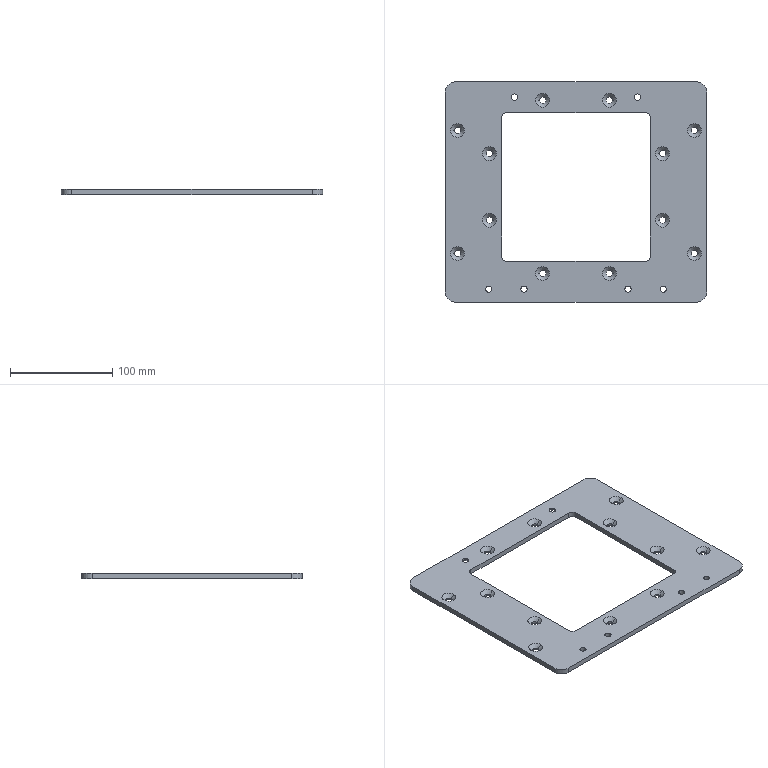NC program | NX | posted with a generic post | part box 255 x 215 x 5 mm
Lines 6275 to 7663 of 7663:
(ZLEVEL_PROFILE_COPY_1_COPY_2 , TOOL : D10JING)
N12512 T14 M6
N12514 G54
N12516 G17 G0 G90 X67.5 Y13.343 S9500 M3
N12518 G43 Z30. H14
N12520 Z1.5
N12522 G94 G1 Y72.494 Z-1.6 F1000.
N12524 X67.454 Y72.5 F1500.
N12526 X-67.41
N12528 X-67.5 Y72.494
N12530 Y-62.41
N12532 X-67.494 Y-62.5
N12534 X67.494
N12536 X67.5 Y-62.454
N12538 Y72.494
N12540 X62.661 Y72.5 Z-1.614
N12542 X-57.777 Z-1.971
N12544 X-62.593 Z-1.985
N12546 X-67.41 Y72.498 Z-2.
N12548 X-67.491 Y72.493
N12550 X-67.496 Y72.424
N12552 X-67.5 Y67.643 Z-2.014
N12554 Y62.858 Z-2.029
N12556 Y-52.774 Z-2.371
N12558 Y-57.592 Z-2.385
N12560 X-67.498 Y-62.41 Z-2.4
N12562 X-67.493 Y-62.491
N12564 X-67.424 Y-62.496
N12566 X-62.64 Y-62.5 Z-2.414
N12568 X-57.852 Z-2.429
N12570 X57.852 Z-2.771
N12572 X62.653 Z-2.786
N12574 X67.492 Y-62.492 Z-2.8
N12576 X67.5 Y-57.635 Z-2.814
N12578 Y-52.815 Z-2.829
N12580 Y67.675 Z-3.186
N12582 Y72.494 Z-3.2
N12584 X62.661 Y72.5 Z-3.214
N12586 X-57.777 Z-3.571
N12588 X-62.593 Z-3.585
N12590 X-67.41 Y72.498 Z-3.6
N12592 X-67.491 Y72.493
N12594 X-67.496 Y72.424
N12596 X-67.5 Y67.643 Z-3.614
N12598 Y62.858 Z-3.629
N12600 Y-52.774 Z-3.971
N12602 Y-57.592 Z-3.985
N12604 X-67.498 Y-62.41 Z-4.
N12606 X-67.493 Y-62.491
N12608 X-67.424 Y-62.496
N12610 X-62.64 Y-62.5 Z-4.014
N12612 X-57.852 Z-4.029
N12614 X57.852 Z-4.371
N12616 X62.653 Z-4.386
N12618 X67.493 Y-62.493 Z-4.4
N12620 X67.5 Y-57.635 Z-4.414
N12622 Y-52.815 Z-4.429
N12624 Y62.855 Z-4.771
N12626 Y67.675 Z-4.786
N12628 Y72.494 Z-4.8
N12630 X67.454 Y72.5
N12632 X-67.41
N12634 X-67.5 Y72.494
N12636 Y-62.41
N12638 X-67.494 Y-62.5
N12640 X67.494
N12642 X67.5 Y-62.454
N12644 Y72.494
N12646 Z-3.3
N12648 G0 Z30.
(ZLEVEL_PROFILE_COPY_1_COPY_COPY , TOOL : D10JING)
N12650 X-119.184 Y114.416
N12652 Z-3.525
N12654 G1 Z-4.525 F1000.
N12656 X-118.366 Y113.
N12658 G3 X-117.5 Y112.5 R1.
N12660 G1 X117.5 F1200.
N12662 G2 X132.5 Y97.5 R15.
N12664 G1 Y-97.5
N12666 G2 X117.5 Y-112.5 R15.
N12668 G1 X-117.5
N12670 G2 X-132.5 Y-97.5 R15.
N12672 G1 Y97.5
N12674 G2 X-117.5 Y112.5 R15.
N12676 G1 X117.43 Z-4.556
N12678 X117.653 Y112.499
N12680 X117.877 Y112.495
N12682 X118.1 Y112.488
N12684 X118.323 Y112.477
N12686 X118.546 Y112.463
N12688 X118.769 Y112.446
N12690 X118.992 Y112.426
N12692 X119.214 Y112.402
N12694 X119.436 Y112.375
N12696 X119.657 Y112.344
N12698 X119.878 Y112.31
N12700 X120.099 Y112.273
N12702 X120.319 Y112.233
N12704 X120.538 Y112.189
N12706 X120.756 Y112.142
N12708 X120.974 Y112.092
N12710 X121.191 Y112.039
N12712 X121.408 Y111.982
N12714 X121.623 Y111.922
N12716 X121.837 Y111.859
N12718 X122.051 Y111.793
N12720 X122.263 Y111.724
N12722 X122.475 Y111.651
N12724 X122.685 Y111.575
N12726 X122.894 Y111.497 Z-4.557
N12728 X123.102 Y111.415
N12730 X123.309 Y111.33
N12732 X123.514 Y111.241
N12734 X123.718 Y111.15
N12736 X123.921 Y111.056
N12738 X124.122 Y110.959
N12740 X124.322 Y110.859
N12742 X124.521 Y110.756
N12744 X124.717 Y110.65
N12746 X124.912 Y110.541
N12748 X125.106 Y110.429
N12750 X125.298 Y110.314
N12752 X125.488 Y110.196
N12754 X125.676 Y110.076
N12756 X125.863 Y109.953
N12758 X126.047 Y109.827
N12760 X126.23 Y109.698
N12762 X126.411 Y109.566
N12764 X126.59 Y109.432
N12766 X126.766 Y109.295
N12768 X126.941 Y109.156
N12770 X127.114 Y109.014
N12772 X127.284 Y108.87
N12774 X127.453 Y108.722
N12776 X127.619 Y108.573
N12778 X127.783 Y108.421
N12780 X127.944 Y108.266
N12782 X128.104 Y108.11
N12784 X128.26 Y107.95
N12786 X128.415 Y107.789
N12788 X128.567 Y107.625
N12790 X128.717 Y107.459
N12792 X128.864 Y107.291
N12794 X129.009 Y107.12 Z-4.558
N12796 X129.151 Y106.948
N12798 X129.29 Y106.773
N12800 X129.427 Y106.597
N12802 X129.561 Y106.418
N12804 X129.693 Y106.237
N12806 X129.822 Y106.054
N12808 X129.948 Y105.87
N12810 X130.071 Y105.683
N12812 X130.192 Y105.495
N12814 X130.309 Y105.305
N12816 X130.424 Y105.113
N12818 X130.536 Y104.92
N12820 X130.645 Y104.725
N12822 X130.752 Y104.528
N12824 X130.855 Y104.33
N12826 X130.955 Y104.13
N12828 X131.052 Y103.929
N12830 X131.147 Y103.726
N12832 X131.238 Y103.522
N12834 X131.326 Y103.317
N12836 X131.411 Y103.11
N12838 X131.493 Y102.902
N12840 X131.572 Y102.693
N12842 X131.648 Y102.483
N12844 X131.721 Y102.272
N12846 X131.79 Y102.059
N12848 X131.857 Y101.846
N12850 X131.92 Y101.631
N12852 X131.98 Y101.416
N12854 X132.037 Y101.2
N12856 X132.09 Y100.983
N12858 X132.14 Y100.765
N12860 X132.187 Y100.546
N12862 X132.231 Y100.327
N12864 X132.272 Y100.107 Z-4.559
N12866 X132.309 Y99.887
N12868 X132.343 Y99.666
N12870 X132.373 Y99.444
N12872 X132.401 Y99.223
N12874 X132.425 Y99.
N12876 X132.445 Y98.778
N12878 X132.463 Y98.555
N12880 X132.477 Y98.332
N12882 X132.488 Y98.109
N12884 X132.495 Y97.885
N12886 X132.499 Y97.662
N12888 X132.5 Y97.438
N12890 Y-97.48 Z-4.584
N12892 X132.499 Y-97.703
N12894 X132.494 Y-97.927
N12896 X132.486 Y-98.15
N12898 X132.475 Y-98.373 Z-4.585
N12900 X132.46 Y-98.596
N12902 X132.442 Y-98.819
N12904 X132.421 Y-99.042
N12906 X132.396 Y-99.264
N12908 X132.368 Y-99.485
N12910 X132.337 Y-99.707
N12912 X132.302 Y-99.928
N12914 X132.264 Y-100.148
N12916 X132.223 Y-100.368
N12918 X132.179 Y-100.587
N12920 X132.131 Y-100.805
N12922 X132.08 Y-101.023
N12924 X132.026 Y-101.24
N12926 X131.969 Y-101.456
N12928 X131.908 Y-101.671
N12930 X131.845 Y-101.885
N12932 X131.778 Y-102.098
N12934 X131.708 Y-102.311
N12936 X131.634 Y-102.522
N12938 X131.558 Y-102.732
N12940 X131.478 Y-102.941
N12942 X131.396 Y-103.149
N12944 X131.31 Y-103.355
N12946 X131.221 Y-103.56
N12948 X131.13 Y-103.764
N12950 X131.035 Y-103.966
N12952 X130.937 Y-104.167
N12954 X130.836 Y-104.367
N12956 X130.732 Y-104.565
N12958 X130.625 Y-104.761
N12960 X130.516 Y-104.956
N12962 X130.403 Y-105.149
N12964 X130.288 Y-105.34
N12966 X130.17 Y-105.53 Z-4.586
N12968 X130.048 Y-105.718
N12970 X129.925 Y-105.904
N12972 X129.798 Y-106.088
N12974 X129.669 Y-106.271
N12976 X129.537 Y-106.451
N12978 X129.402 Y-106.629
N12980 X129.265 Y-106.806
N12982 X129.125 Y-106.98
N12984 X128.982 Y-107.152
N12986 X128.837 Y-107.322
N12988 X128.689 Y-107.49
N12990 X128.539 Y-107.656
N12992 X128.387 Y-107.819
N12994 X128.232 Y-107.98
N12996 X128.074 Y-108.139
N12998 X127.915 Y-108.295
N13000 X127.753 Y-108.449
N13002 X127.588 Y-108.601
N13004 X127.422 Y-108.75
N13006 X127.253 Y-108.896
N13008 X127.082 Y-109.041
N13010 X126.909 Y-109.182
N13012 X126.734 Y-109.321
N13014 X126.557 Y-109.457
N13016 X126.378 Y-109.591
N13018 X126.196 Y-109.722
N13020 X126.013 Y-109.85
N13022 X125.828 Y-109.976
N13024 X125.641 Y-110.098
N13026 X125.453 Y-110.218
N13028 X125.262 Y-110.335
N13030 X125.07 Y-110.45
N13032 X124.877 Y-110.561
N13034 X124.681 Y-110.669 Z-4.587
N13036 X124.484 Y-110.775
N13038 X124.285 Y-110.878
N13040 X124.085 Y-110.977
N13042 X123.884 Y-111.074
N13044 X123.681 Y-111.167
N13046 X123.476 Y-111.258
N13048 X123.271 Y-111.346
N13050 X123.064 Y-111.43
N13052 X122.856 Y-111.511
N13054 X122.646 Y-111.59
N13056 X122.436 Y-111.665
N13058 X122.224 Y-111.737
N13060 X122.011 Y-111.805
N13062 X121.798 Y-111.871
N13064 X121.583 Y-111.934
N13066 X121.368 Y-111.993
N13068 X121.151 Y-112.049
N13070 X120.934 Y-112.102
N13072 X120.716 Y-112.151
N13074 X120.497 Y-112.197
N13076 X120.278 Y-112.241
N13078 X120.058 Y-112.28
N13080 X119.837 Y-112.317
N13082 X119.616 Y-112.35
N13084 X119.395 Y-112.38
N13086 X119.173 Y-112.406
N13088 X118.951 Y-112.43
N13090 X118.728 Y-112.45
N13092 X118.505 Y-112.466
N13094 X118.282 Y-112.48
N13096 X118.059 Y-112.49
N13098 X117.835 Y-112.496
N13100 X117.612 Y-112.5
N13102 X117.388 Z-4.588
N13104 X-117.318 Z-4.618
N13106 X-117.541
N13108 X-117.765 Y-112.498
N13110 X-117.988 Y-112.492
N13112 X-118.212 Y-112.483
N13114 X-118.435 Y-112.471
N13116 X-118.658 Y-112.455
N13118 X-118.881 Y-112.436
N13120 X-119.103 Y-112.414
N13122 X-119.325 Y-112.389 Z-4.619
N13124 X-119.547 Y-112.36
N13126 X-119.768 Y-112.328
N13128 X-119.989 Y-112.292
N13130 X-120.209 Y-112.253
N13132 X-120.428 Y-112.211
N13134 X-120.647 Y-112.166
N13136 X-120.865 Y-112.118
N13138 X-121.083 Y-112.066
N13140 X-121.3 Y-112.011
N13142 X-121.515 Y-111.953
N13144 X-121.73 Y-111.891
N13146 X-121.944 Y-111.827
N13148 X-122.157 Y-111.759
N13150 X-122.369 Y-111.688
N13152 X-122.58 Y-111.614
N13154 X-122.79 Y-111.536
N13156 X-122.998 Y-111.456
N13158 X-123.206 Y-111.372
N13160 X-123.412 Y-111.286
N13162 X-123.617 Y-111.196
N13164 X-123.82 Y-111.104
N13166 X-124.022 Y-111.008
N13168 X-124.223 Y-110.909
N13170 X-124.422 Y-110.808
N13172 X-124.619 Y-110.703
N13174 X-124.815 Y-110.595
N13176 X-125.009 Y-110.485
N13178 X-125.202 Y-110.372
N13180 X-125.393 Y-110.255
N13182 X-125.582 Y-110.136
N13184 X-125.77 Y-110.015
N13186 X-125.955 Y-109.89
N13188 X-126.139 Y-109.763
N13190 X-126.321 Y-109.632 Z-4.62
N13192 X-126.5 Y-109.5
N13194 X-126.678 Y-109.364
N13196 X-126.854 Y-109.226
N13198 X-127.028 Y-109.085
N13200 X-127.199 Y-108.942
N13202 X-127.369 Y-108.796
N13204 X-127.536 Y-108.648
N13206 X-127.701 Y-108.497
N13208 X-127.864 Y-108.344
N13210 X-128.024 Y-108.188
N13212 X-128.182 Y-108.03
N13214 X-128.338 Y-107.87
N13216 X-128.491 Y-107.707
N13218 X-128.642 Y-107.542
N13220 X-128.791 Y-107.375
N13222 X-128.937 Y-107.206
N13224 X-129.08 Y-107.034
N13226 X-129.221 Y-106.861
N13228 X-129.359 Y-106.685
N13230 X-129.494 Y-106.507
N13232 X-129.627 Y-106.328
N13234 X-129.758 Y-106.146
N13236 X-129.885 Y-105.962
N13238 X-130.01 Y-105.777
N13240 X-130.132 Y-105.59
N13242 X-130.251 Y-105.4
N13244 X-130.367 Y-105.21
N13246 X-130.481 Y-105.017
N13248 X-130.591 Y-104.823
N13250 X-130.699 Y-104.627
N13252 X-130.804 Y-104.429
N13254 X-130.905 Y-104.23
N13256 X-131.004 Y-104.03
N13258 X-131.1 Y-103.828 Z-4.621
N13260 X-131.193 Y-103.624
N13262 X-131.282 Y-103.42
N13264 X-131.369 Y-103.214
N13266 X-131.453 Y-103.006
N13268 X-131.533 Y-102.798
N13270 X-131.611 Y-102.588
N13272 X-131.685 Y-102.377
N13274 X-131.756 Y-102.165
N13276 X-131.824 Y-101.952
N13278 X-131.889 Y-101.739
N13280 X-131.95 Y-101.524
N13282 X-132.009 Y-101.308
N13284 X-132.064 Y-101.091
N13286 X-132.116 Y-100.874
N13288 X-132.164 Y-100.656
N13290 X-132.21 Y-100.437
N13292 X-132.252 Y-100.217
N13294 X-132.291 Y-99.997
N13296 X-132.326 Y-99.776
N13298 X-132.359 Y-99.555
N13300 X-132.388 Y-99.334
N13302 X-132.413 Y-99.112
N13304 X-132.436 Y-98.889
N13306 X-132.455 Y-98.666
N13308 X-132.47 Y-98.443
N13310 X-132.483 Y-98.22
N13312 X-132.492 Y-97.997
N13314 X-132.498 Y-97.774
N13316 X-132.5 Y-97.55
N13318 Y-97.326
N13320 Y97.368 Z-4.647
N13322 Y97.591
N13324 X-132.497 Y97.815
N13326 X-132.49 Y98.038
N13328 X-132.481 Y98.262
N13330 X-132.468 Y98.485
N13332 X-132.451 Y98.708
N13334 X-132.432 Y98.93
N13336 X-132.409 Y99.153
N13338 X-132.382 Y99.375
N13340 X-132.353 Y99.596
N13342 X-132.32 Y99.817
N13344 X-132.284 Y100.038
N13346 X-132.244 Y100.258
N13348 X-132.202 Y100.477
N13350 X-132.156 Y100.696
N13352 X-132.106 Y100.914
N13354 X-132.054 Y101.131
N13356 X-131.998 Y101.348
N13358 X-131.939 Y101.563
N13360 X-131.877 Y101.778
N13362 X-131.812 Y101.992 Z-4.648
N13364 X-131.743 Y102.205
N13366 X-131.671 Y102.416
N13368 X-131.597 Y102.627
N13370 X-131.519 Y102.837
N13372 X-131.438 Y103.045
N13374 X-131.353 Y103.252
N13376 X-131.266 Y103.458
N13378 X-131.176 Y103.662
N13380 X-131.082 Y103.865
N13382 X-130.986 Y104.067
N13384 X-130.887 Y104.267
N13386 X-130.784 Y104.466
N13388 X-130.679 Y104.663
N13390 X-130.571 Y104.859
N13392 X-130.46 Y105.053
N13394 X-130.346 Y105.245
N13396 X-130.229 Y105.436
N13398 X-130.109 Y105.624
N13400 X-129.987 Y105.811
N13402 X-129.862 Y105.996
N13404 X-129.734 Y106.18
N13406 X-129.603 Y106.361
N13408 X-129.47 Y106.54
N13410 X-129.334 Y106.718
N13412 X-129.195 Y106.893
N13414 X-129.054 Y107.066
N13416 X-128.91 Y107.237
N13418 X-128.763 Y107.406
N13420 X-128.615 Y107.573
N13422 X-128.463 Y107.738
N13424 X-128.309 Y107.9
N13426 X-128.153 Y108.06
N13428 X-127.995 Y108.217
N13430 X-127.834 Y108.373 Z-4.649
N13432 X-127.671 Y108.525
N13434 X-127.505 Y108.676
N13436 X-127.338 Y108.824
N13438 X-127.168 Y108.969
N13440 X-126.996 Y109.112
N13442 X-126.822 Y109.252
N13444 X-126.646 Y109.389
N13446 X-126.467 Y109.524
N13448 X-126.287 Y109.657
N13450 X-126.105 Y109.786
N13452 X-125.921 Y109.913
N13454 X-125.735 Y110.037
N13456 X-125.547 Y110.159
N13458 X-125.358 Y110.277
N13460 X-125.167 Y110.393
N13462 X-124.974 Y110.506
N13464 X-124.779 Y110.616
N13466 X-124.583 Y110.723
N13468 X-124.385 Y110.827
N13470 X-124.186 Y110.928
N13472 X-123.985 Y111.026
N13474 X-123.782 Y111.121
N13476 X-123.579 Y111.213
N13478 X-123.374 Y111.302
N13480 X-123.167 Y111.388
N13482 X-122.96 Y111.471
N13484 X-122.751 Y111.551
N13486 X-122.541 Y111.628
N13488 X-122.33 Y111.701
N13490 X-122.118 Y111.771
N13492 X-121.905 Y111.839
N13494 X-121.691 Y111.903
N13496 X-121.475 Y111.964
N13498 X-121.259 Y112.021 Z-4.65
N13500 X-121.043 Y112.076
N13502 X-120.825 Y112.127
N13504 X-120.607 Y112.175
N13506 X-120.388 Y112.219
N13508 X-120.168 Y112.261
N13510 X-119.948 Y112.299
N13512 X-119.727 Y112.334
N13514 X-119.506 Y112.365
N13516 X-119.284 Y112.394
N13518 X-119.062 Y112.418
N13520 X-118.839 Y112.44
N13522 X-118.617 Y112.458
N13524 X-118.394 Y112.473
N13526 X-118.17 Y112.485
N13528 X-117.947 Y112.493
N13530 X-117.724 Y112.498
N13532 X-117.5 Y112.5
N13534 X117.43 Z-4.681
N13536 X117.653 Y112.499
N13538 X117.877 Y112.495
N13540 X118.1 Y112.488
N13542 X118.323 Y112.477
N13544 X118.546 Y112.463
N13546 X118.769 Y112.446
N13548 X118.992 Y112.426
N13550 X119.214 Y112.402
N13552 X119.436 Y112.375
N13554 X119.657 Y112.344
N13556 X119.878 Y112.31
N13558 X120.099 Y112.273
N13560 X120.319 Y112.233
N13562 X120.538 Y112.189
N13564 X120.756 Y112.142
N13566 X120.974 Y112.092
N13568 X121.191 Y112.039
N13570 X121.408 Y111.982
N13572 X121.623 Y111.922
N13574 X121.837 Y111.859
N13576 X122.051 Y111.793
N13578 X122.263 Y111.724
N13580 X122.475 Y111.651
N13582 X122.685 Y111.575
N13584 X122.894 Y111.497 Z-4.682
N13586 X123.102 Y111.415
N13588 X123.309 Y111.33
N13590 X123.514 Y111.241
N13592 X123.718 Y111.15
N13594 X123.921 Y111.056
N13596 X124.122 Y110.959
N13598 X124.322 Y110.859
N13600 X124.521 Y110.756
N13602 X124.717 Y110.65
N13604 X124.912 Y110.541
N13606 X125.106 Y110.429
N13608 X125.298 Y110.314
N13610 X125.488 Y110.196
N13612 X125.676 Y110.076
N13614 X125.863 Y109.953
N13616 X126.047 Y109.827
N13618 X126.23 Y109.698
N13620 X126.411 Y109.566
N13622 X126.59 Y109.432
N13624 X126.766 Y109.295
N13626 X126.941 Y109.156
N13628 X127.114 Y109.014
N13630 X127.284 Y108.87
N13632 X127.453 Y108.722
N13634 X127.619 Y108.573
N13636 X127.783 Y108.421
N13638 X127.944 Y108.266
N13640 X128.104 Y108.11
N13642 X128.26 Y107.95
N13644 X128.415 Y107.789
N13646 X128.567 Y107.625
N13648 X128.717 Y107.459
N13650 X128.864 Y107.291
N13652 X129.009 Y107.12 Z-4.683
N13654 X129.151 Y106.948
N13656 X129.29 Y106.773
N13658 X129.427 Y106.597
N13660 X129.561 Y106.418
N13662 X129.693 Y106.237
N13664 X129.822 Y106.054
N13666 X129.948 Y105.87
N13668 X130.071 Y105.683
N13670 X130.192 Y105.495
N13672 X130.309 Y105.305
N13674 X130.424 Y105.113
N13676 X130.536 Y104.92
N13678 X130.645 Y104.725
N13680 X130.752 Y104.528
N13682 X130.855 Y104.33
N13684 X130.955 Y104.13
N13686 X131.052 Y103.929
N13688 X131.147 Y103.726
N13690 X131.238 Y103.522
N13692 X131.326 Y103.317
N13694 X131.411 Y103.11
N13696 X131.493 Y102.902
N13698 X131.572 Y102.693
N13700 X131.648 Y102.483
N13702 X131.721 Y102.272
N13704 X131.79 Y102.059
N13706 X131.857 Y101.846
N13708 X131.92 Y101.631
N13710 X131.98 Y101.416
N13712 X132.037 Y101.2
N13714 X132.09 Y100.983
N13716 X132.14 Y100.765
N13718 X132.187 Y100.546
N13720 X132.231 Y100.327
N13722 X132.272 Y100.107 Z-4.684
N13724 X132.309 Y99.887
N13726 X132.343 Y99.666
N13728 X132.373 Y99.444
N13730 X132.401 Y99.223
N13732 X132.425 Y99.
N13734 X132.445 Y98.778
N13736 X132.463 Y98.555
N13738 X132.477 Y98.332
N13740 X132.488 Y98.109
N13742 X132.495 Y97.885
N13744 X132.499 Y97.662
N13746 X132.5 Y97.438
N13748 Y-97.48 Z-4.709
N13750 X132.499 Y-97.703
N13752 X132.494 Y-97.927
N13754 X132.486 Y-98.15
N13756 X132.475 Y-98.373 Z-4.71
N13758 X132.46 Y-98.596
N13760 X132.442 Y-98.819
N13762 X132.421 Y-99.042
N13764 X132.396 Y-99.264
N13766 X132.368 Y-99.485
N13768 X132.337 Y-99.707
N13770 X132.302 Y-99.928
N13772 X132.264 Y-100.148
N13774 X132.223 Y-100.368
N13776 X132.179 Y-100.587
N13778 X132.131 Y-100.805
N13780 X132.08 Y-101.023
N13782 X132.026 Y-101.24
N13784 X131.969 Y-101.456
N13786 X131.908 Y-101.671
N13788 X131.845 Y-101.885
N13790 X131.778 Y-102.098
N13792 X131.708 Y-102.311
N13794 X131.634 Y-102.522
N13796 X131.558 Y-102.732
N13798 X131.478 Y-102.941
N13800 X131.396 Y-103.149
N13802 X131.31 Y-103.355
N13804 X131.221 Y-103.56
N13806 X131.13 Y-103.764
N13808 X131.035 Y-103.966
N13810 X130.937 Y-104.167
N13812 X130.836 Y-104.367
N13814 X130.732 Y-104.565
N13816 X130.625 Y-104.761
N13818 X130.516 Y-104.956
N13820 X130.403 Y-105.149
N13822 X130.288 Y-105.34
N13824 X130.17 Y-105.53 Z-4.711
N13826 X130.048 Y-105.718
N13828 X129.925 Y-105.904
N13830 X129.798 Y-106.088
N13832 X129.669 Y-106.271
N13834 X129.537 Y-106.451
N13836 X129.402 Y-106.629
N13838 X129.265 Y-106.806
N13840 X129.125 Y-106.98
N13842 X128.982 Y-107.152
N13844 X128.837 Y-107.322
N13846 X128.689 Y-107.49
N13848 X128.539 Y-107.656
N13850 X128.387 Y-107.819
N13852 X128.232 Y-107.98
N13854 X128.074 Y-108.139
N13856 X127.915 Y-108.295
N13858 X127.753 Y-108.449
N13860 X127.588 Y-108.601
N13862 X127.422 Y-108.75
N13864 X127.253 Y-108.896
N13866 X127.082 Y-109.041
N13868 X126.909 Y-109.182
N13870 X126.734 Y-109.321
N13872 X126.557 Y-109.457
N13874 X126.378 Y-109.591
N13876 X126.196 Y-109.722
N13878 X126.013 Y-109.85
N13880 X125.828 Y-109.976
N13882 X125.641 Y-110.098
N13884 X125.453 Y-110.218
N13886 X125.262 Y-110.335
N13888 X125.07 Y-110.45
N13890 X124.877 Y-110.561
N13892 X124.681 Y-110.669 Z-4.712
N13894 X124.484 Y-110.775
N13896 X124.285 Y-110.878
N13898 X124.085 Y-110.977
N13900 X123.884 Y-111.074
N13902 X123.681 Y-111.167
N13904 X123.476 Y-111.258
N13906 X123.271 Y-111.346
N13908 X123.064 Y-111.43
N13910 X122.856 Y-111.511
N13912 X122.646 Y-111.59
N13914 X122.436 Y-111.665
N13916 X122.224 Y-111.737
N13918 X122.011 Y-111.805
N13920 X121.798 Y-111.871
N13922 X121.583 Y-111.934
N13924 X121.368 Y-111.993
N13926 X121.151 Y-112.049
N13928 X120.934 Y-112.102
N13930 X120.716 Y-112.151
N13932 X120.497 Y-112.197
N13934 X120.278 Y-112.241
N13936 X120.058 Y-112.28
N13938 X119.837 Y-112.317
N13940 X119.616 Y-112.35
N13942 X119.395 Y-112.38
N13944 X119.173 Y-112.406
N13946 X118.951 Y-112.43
N13948 X118.728 Y-112.45
N13950 X118.505 Y-112.466
N13952 X118.282 Y-112.48
N13954 X118.059 Y-112.49
N13956 X117.835 Y-112.496
N13958 X117.612 Y-112.5
N13960 X117.388 Z-4.713
N13962 X-117.318 Z-4.743
N13964 X-117.541
N13966 X-117.765 Y-112.498
N13968 X-117.988 Y-112.492
N13970 X-118.212 Y-112.483
N13972 X-118.435 Y-112.471
N13974 X-118.658 Y-112.455
N13976 X-118.881 Y-112.436
N13978 X-119.103 Y-112.414
N13980 X-119.325 Y-112.389 Z-4.744
N13982 X-119.547 Y-112.36
N13984 X-119.768 Y-112.328
N13986 X-119.989 Y-112.292
N13988 X-120.209 Y-112.253
N13990 X-120.428 Y-112.211
N13992 X-120.647 Y-112.166
N13994 X-120.865 Y-112.118
N13996 X-121.083 Y-112.066
N13998 X-121.3 Y-112.011
N14000 X-121.515 Y-111.953
N14002 X-121.73 Y-111.891
N14004 X-121.944 Y-111.827
N14006 X-122.157 Y-111.759
N14008 X-122.369 Y-111.688
N14010 X-122.58 Y-111.614
N14012 X-122.79 Y-111.536
N14014 X-122.998 Y-111.456
N14016 X-123.206 Y-111.372
N14018 X-123.412 Y-111.286
N14020 X-123.617 Y-111.196
N14022 X-123.82 Y-111.104
N14024 X-124.022 Y-111.008
N14026 X-124.223 Y-110.909
N14028 X-124.422 Y-110.808
N14030 X-124.619 Y-110.703
N14032 X-124.815 Y-110.595
N14034 X-125.009 Y-110.485
N14036 X-125.202 Y-110.372
N14038 X-125.393 Y-110.255
N14040 X-125.582 Y-110.136
N14042 X-125.77 Y-110.015
N14044 X-125.955 Y-109.89
N14046 X-126.139 Y-109.763
N14048 X-126.321 Y-109.632 Z-4.745
N14050 X-126.5 Y-109.5
N14052 X-126.678 Y-109.364
N14054 X-126.854 Y-109.226
N14056 X-127.028 Y-109.085
N14058 X-127.199 Y-108.942
N14060 X-127.369 Y-108.796
N14062 X-127.536 Y-108.648
N14064 X-127.701 Y-108.497
N14066 X-127.864 Y-108.344
N14068 X-128.024 Y-108.188
N14070 X-128.182 Y-108.03
N14072 X-128.338 Y-107.87
N14074 X-128.491 Y-107.707
N14076 X-128.642 Y-107.542
N14078 X-128.791 Y-107.375
N14080 X-128.937 Y-107.206
N14082 X-129.08 Y-107.034
N14084 X-129.221 Y-106.861
N14086 X-129.359 Y-106.685
N14088 X-129.494 Y-106.507
N14090 X-129.627 Y-106.328
N14092 X-129.758 Y-106.146
N14094 X-129.885 Y-105.962
N14096 X-130.01 Y-105.777
N14098 X-130.132 Y-105.59
N14100 X-130.251 Y-105.4
N14102 X-130.367 Y-105.21
N14104 X-130.481 Y-105.017
N14106 X-130.591 Y-104.823
N14108 X-130.699 Y-104.627
N14110 X-130.804 Y-104.429
N14112 X-130.905 Y-104.23
N14114 X-131.004 Y-104.03
N14116 X-131.1 Y-103.828 Z-4.746
N14118 X-131.193 Y-103.624
N14120 X-131.282 Y-103.42
N14122 X-131.369 Y-103.214
N14124 X-131.453 Y-103.006
N14126 X-131.533 Y-102.798
N14128 X-131.611 Y-102.588
N14130 X-131.685 Y-102.377
N14132 X-131.756 Y-102.165
N14134 X-131.824 Y-101.952
N14136 X-131.889 Y-101.739
N14138 X-131.95 Y-101.524
N14140 X-132.009 Y-101.308
N14142 X-132.064 Y-101.091
N14144 X-132.116 Y-100.874
N14146 X-132.164 Y-100.656
N14148 X-132.21 Y-100.437
N14150 X-132.252 Y-100.217
N14152 X-132.291 Y-99.997
N14154 X-132.326 Y-99.776
N14156 X-132.359 Y-99.555
N14158 X-132.388 Y-99.334
N14160 X-132.413 Y-99.112
N14162 X-132.436 Y-98.889
N14164 X-132.455 Y-98.666
N14166 X-132.47 Y-98.443
N14168 X-132.483 Y-98.22
N14170 X-132.492 Y-97.997
N14172 X-132.498 Y-97.774
N14174 X-132.5 Y-97.55
N14176 Y-97.326
N14178 Y97.368 Z-4.772
N14180 Y97.591
N14182 X-132.497 Y97.815
N14184 X-132.49 Y98.038
N14186 X-132.481 Y98.262
N14188 X-132.468 Y98.485
N14190 X-132.451 Y98.708
N14192 X-132.432 Y98.93
N14194 X-132.409 Y99.153
N14196 X-132.382 Y99.375
N14198 X-132.353 Y99.596
N14200 X-132.32 Y99.817
N14202 X-132.284 Y100.038
N14204 X-132.244 Y100.258
N14206 X-132.202 Y100.477
N14208 X-132.156 Y100.696
N14210 X-132.106 Y100.914
N14212 X-132.054 Y101.131
N14214 X-131.998 Y101.348
N14216 X-131.939 Y101.563
N14218 X-131.877 Y101.778
N14220 X-131.812 Y101.992 Z-4.773
N14222 X-131.743 Y102.205
N14224 X-131.671 Y102.416
N14226 X-131.597 Y102.627
N14228 X-131.519 Y102.837
N14230 X-131.438 Y103.045
N14232 X-131.353 Y103.252
N14234 X-131.266 Y103.458
N14236 X-131.176 Y103.662
N14238 X-131.082 Y103.865
N14240 X-130.986 Y104.067
N14242 X-130.887 Y104.267
N14244 X-130.784 Y104.466
N14246 X-130.679 Y104.663
N14248 X-130.571 Y104.859
N14250 X-130.46 Y105.053
N14252 X-130.346 Y105.245
N14254 X-130.229 Y105.436
N14256 X-130.109 Y105.624
N14258 X-129.987 Y105.811
N14260 X-129.862 Y105.996
N14262 X-129.734 Y106.18
N14264 X-129.603 Y106.361
N14266 X-129.47 Y106.54
N14268 X-129.334 Y106.718
N14270 X-129.195 Y106.893
N14272 X-129.054 Y107.066
N14274 X-128.91 Y107.237
N14276 X-128.763 Y107.406
N14278 X-128.615 Y107.573
N14280 X-128.463 Y107.738
N14282 X-128.309 Y107.9
N14284 X-128.153 Y108.06
N14286 X-127.995 Y108.217
N14288 X-127.834 Y108.373 Z-4.774
N14290 X-127.671 Y108.525
N14292 X-127.505 Y108.676
N14294 X-127.338 Y108.824
N14296 X-127.168 Y108.969
N14298 X-126.996 Y109.112
N14300 X-126.822 Y109.252
N14302 X-126.646 Y109.389
N14304 X-126.467 Y109.524
N14306 X-126.287 Y109.657
N14308 X-126.105 Y109.786
N14310 X-125.921 Y109.913
N14312 X-125.735 Y110.037
N14314 X-125.547 Y110.159
N14316 X-125.358 Y110.277
N14318 X-125.167 Y110.393
N14320 X-124.974 Y110.506
N14322 X-124.779 Y110.616
N14324 X-124.583 Y110.723
N14326 X-124.385 Y110.827
N14328 X-124.186 Y110.928
N14330 X-123.985 Y111.026
N14332 X-123.782 Y111.121
N14334 X-123.579 Y111.213
N14336 X-123.374 Y111.302
N14338 X-123.167 Y111.388
N14340 X-122.96 Y111.471
N14342 X-122.751 Y111.551
N14344 X-122.541 Y111.628
N14346 X-122.33 Y111.701
N14348 X-122.118 Y111.771
N14350 X-121.905 Y111.839
N14352 X-121.691 Y111.903
N14354 X-121.475 Y111.964
N14356 X-121.259 Y112.021 Z-4.775
N14358 X-121.043 Y112.076
N14360 X-120.825 Y112.127
N14362 X-120.607 Y112.175
N14364 X-120.388 Y112.219
N14366 X-120.168 Y112.261
N14368 X-119.948 Y112.299
N14370 X-119.727 Y112.334
N14372 X-119.506 Y112.365
N14374 X-119.284 Y112.394
N14376 X-119.062 Y112.418
N14378 X-118.839 Y112.44
N14380 X-118.617 Y112.458
N14382 X-118.394 Y112.473
N14384 X-118.17 Y112.485
N14386 X-117.947 Y112.493
N14388 X-117.724 Y112.498
N14390 X-117.5 Y112.5
N14392 X117.43 Z-4.806
N14394 X117.653 Y112.499
N14396 X117.877 Y112.495
N14398 X118.1 Y112.488
N14400 X118.323 Y112.477
N14402 X118.546 Y112.463
N14404 X118.769 Y112.446
N14406 X118.992 Y112.426
N14408 X119.214 Y112.402
N14410 X119.436 Y112.375
N14412 X119.657 Y112.344
N14414 X119.878 Y112.31
N14416 X120.099 Y112.273
N14418 X120.319 Y112.233
N14420 X120.538 Y112.189
N14422 X120.756 Y112.142
N14424 X120.974 Y112.092
N14426 X121.191 Y112.039
N14428 X121.408 Y111.982
N14430 X121.623 Y111.922
N14432 X121.837 Y111.859
N14434 X122.051 Y111.793
N14436 X122.263 Y111.724
N14438 X122.475 Y111.651
N14440 X122.685 Y111.575
N14442 X122.894 Y111.497 Z-4.807
N14444 X123.102 Y111.415
N14446 X123.309 Y111.33
N14448 X123.514 Y111.241
N14450 X123.718 Y111.15
N14452 X123.921 Y111.056
N14454 X124.122 Y110.959
N14456 X124.322 Y110.859
N14458 X124.521 Y110.756
N14460 X124.717 Y110.65
N14462 X124.912 Y110.541
N14464 X125.106 Y110.429
N14466 X125.298 Y110.314
N14468 X125.488 Y110.196
N14470 X125.676 Y110.076
N14472 X125.863 Y109.953
N14474 X126.047 Y109.827
N14476 X126.23 Y109.698
N14478 X126.411 Y109.566
N14480 X126.59 Y109.432
N14482 X126.766 Y109.295
N14484 X126.941 Y109.156
N14486 X127.114 Y109.014
N14488 X127.284 Y108.87
N14490 X127.453 Y108.722
N14492 X127.619 Y108.573
N14494 X127.783 Y108.421
N14496 X127.944 Y108.266
N14498 X128.104 Y108.11
N14500 X128.26 Y107.95
N14502 X128.415 Y107.789
N14504 X128.567 Y107.625
N14506 X128.717 Y107.459
N14508 X128.864 Y107.291
N14510 X129.009 Y107.12 Z-4.808
N14512 X129.151 Y106.948
N14514 X129.29 Y106.773
N14516 X129.427 Y106.597
N14518 X129.561 Y106.418
N14520 X129.693 Y106.237
N14522 X129.822 Y106.054
N14524 X129.948 Y105.87
N14526 X130.071 Y105.683
N14528 X130.192 Y105.495
N14530 X130.309 Y105.305
N14532 X130.424 Y105.113
N14534 X130.536 Y104.92
N14536 X130.645 Y104.725
N14538 X130.752 Y104.528
N14540 X130.855 Y104.33
N14542 X130.955 Y104.13
N14544 X131.052 Y103.929
N14546 X131.147 Y103.726
N14548 X131.238 Y103.522
N14550 X131.326 Y103.317
N14552 X131.411 Y103.11
N14554 X131.493 Y102.902
N14556 X131.572 Y102.693
N14558 X131.648 Y102.483
N14560 X131.721 Y102.272
N14562 X131.79 Y102.059
N14564 X131.857 Y101.846
N14566 X131.92 Y101.631
N14568 X131.98 Y101.416
N14570 X132.037 Y101.2
N14572 X132.09 Y100.983
N14574 X132.14 Y100.765
N14576 X132.187 Y100.546
N14578 X132.231 Y100.327
N14580 X132.272 Y100.107 Z-4.809
N14582 X132.309 Y99.887
N14584 X132.343 Y99.666
N14586 X132.373 Y99.444
N14588 X132.401 Y99.223
N14590 X132.425 Y99.
N14592 X132.445 Y98.778
N14594 X132.463 Y98.555
N14596 X132.477 Y98.332
N14598 X132.488 Y98.109
N14600 X132.495 Y97.885
N14602 X132.499 Y97.662
N14604 X132.5 Y97.438
N14606 Y-97.48 Z-4.834
N14608 X132.499 Y-97.703
N14610 X132.494 Y-97.927
N14612 X132.486 Y-98.15
N14614 X132.475 Y-98.373 Z-4.835
N14616 X132.46 Y-98.596
N14618 X132.442 Y-98.819
N14620 X132.421 Y-99.042
N14622 X132.396 Y-99.264
N14624 X132.368 Y-99.485
N14626 X132.337 Y-99.707
N14628 X132.302 Y-99.928
N14630 X132.264 Y-100.148
N14632 X132.223 Y-100.368
N14634 X132.179 Y-100.587
N14636 X132.131 Y-100.805
N14638 X132.08 Y-101.023
N14640 X132.026 Y-101.24
N14642 X131.969 Y-101.456
N14644 X131.908 Y-101.671
N14646 X131.845 Y-101.885
N14648 X131.778 Y-102.098
N14650 X131.708 Y-102.311
N14652 X131.634 Y-102.522
N14654 X131.558 Y-102.732
N14656 X131.478 Y-102.941
N14658 X131.396 Y-103.149
N14660 X131.31 Y-103.355
N14662 X131.221 Y-103.56
N14664 X131.13 Y-103.764
N14666 X131.035 Y-103.966
N14668 X130.937 Y-104.167
N14670 X130.836 Y-104.367
N14672 X130.732 Y-104.565
N14674 X130.625 Y-104.761
N14676 X130.516 Y-104.956
N14678 X130.403 Y-105.149
N14680 X130.288 Y-105.34
N14682 X130.17 Y-105.53 Z-4.836
N14684 X130.048 Y-105.718
N14686 X129.925 Y-105.904
N14688 X129.798 Y-106.088
N14690 X129.669 Y-106.271
N14692 X129.537 Y-106.451
N14694 X129.402 Y-106.629
N14696 X129.265 Y-106.806
N14698 X129.125 Y-106.98
N14700 X128.982 Y-107.152
N14702 X128.837 Y-107.322
N14704 X128.689 Y-107.49
N14706 X128.539 Y-107.656
N14708 X128.387 Y-107.819
N14710 X128.232 Y-107.98
N14712 X128.074 Y-108.139
N14714 X127.915 Y-108.295
N14716 X127.753 Y-108.449
N14718 X127.588 Y-108.601
N14720 X127.422 Y-108.75
N14722 X127.253 Y-108.896
N14724 X127.082 Y-109.041
N14726 X126.909 Y-109.182
N14728 X126.734 Y-109.321
N14730 X126.557 Y-109.457
N14732 X126.378 Y-109.591
N14734 X126.196 Y-109.722
N14736 X126.013 Y-109.85
N14738 X125.828 Y-109.976
N14740 X125.641 Y-110.098
N14742 X125.453 Y-110.218
N14744 X125.262 Y-110.335
N14746 X125.07 Y-110.45
N14748 X124.877 Y-110.561
N14750 X124.681 Y-110.669 Z-4.837
N14752 X124.484 Y-110.775
N14754 X124.285 Y-110.878
N14756 X124.085 Y-110.977
N14758 X123.884 Y-111.074
N14760 X123.681 Y-111.167
N14762 X123.476 Y-111.258
N14764 X123.271 Y-111.346
N14766 X123.064 Y-111.43
N14768 X122.856 Y-111.511
N14770 X122.646 Y-111.59
N14772 X122.436 Y-111.665
N14774 X122.224 Y-111.737
N14776 X122.011 Y-111.805
N14778 X121.798 Y-111.871
N14780 X121.583 Y-111.934
N14782 X121.368 Y-111.993
N14784 X121.151 Y-112.049
N14786 X120.934 Y-112.102
N14788 X120.716 Y-112.151
N14790 X120.497 Y-112.197
N14792 X120.278 Y-112.241
N14794 X120.058 Y-112.28
N14796 X119.837 Y-112.317
N14798 X119.616 Y-112.35
N14800 X119.395 Y-112.38
N14802 X119.173 Y-112.406
N14804 X118.951 Y-112.43
N14806 X118.728 Y-112.45
N14808 X118.505 Y-112.466
N14810 X118.282 Y-112.48
N14812 X118.059 Y-112.49
N14814 X117.835 Y-112.496
N14816 X117.612 Y-112.5
N14818 X117.388 Z-4.838
N14820 X-117.318 Z-4.868
N14822 X-117.541
N14824 X-117.765 Y-112.498
N14826 X-117.988 Y-112.492
N14828 X-118.212 Y-112.483
N14830 X-118.435 Y-112.471
N14832 X-118.658 Y-112.455
N14834 X-118.881 Y-112.436
N14836 X-119.103 Y-112.414
N14838 X-119.325 Y-112.389 Z-4.869
N14840 X-119.547 Y-112.36
N14842 X-119.768 Y-112.328
N14844 X-119.989 Y-112.292
N14846 X-120.209 Y-112.253
N14848 X-120.428 Y-112.211
N14850 X-120.647 Y-112.166
N14852 X-120.865 Y-112.118
N14854 X-121.083 Y-112.066
N14856 X-121.3 Y-112.011
N14858 X-121.515 Y-111.953
N14860 X-121.73 Y-111.891
N14862 X-121.944 Y-111.827
N14864 X-122.157 Y-111.759
N14866 X-122.369 Y-111.688
N14868 X-122.58 Y-111.614
N14870 X-122.79 Y-111.536
N14872 X-122.998 Y-111.456
N14874 X-123.206 Y-111.372
N14876 X-123.412 Y-111.286
N14878 X-123.617 Y-111.196
N14880 X-123.82 Y-111.104
N14882 X-124.022 Y-111.008
N14884 X-124.223 Y-110.909
N14886 X-124.422 Y-110.808
N14888 X-124.619 Y-110.703
N14890 X-124.815 Y-110.595
N14892 X-125.009 Y-110.485
N14894 X-125.202 Y-110.372
N14896 X-125.393 Y-110.255
N14898 X-125.582 Y-110.136
N14900 X-125.77 Y-110.015
N14902 X-125.955 Y-109.89
N14904 X-126.139 Y-109.763
N14906 X-126.321 Y-109.632 Z-4.87
N14908 X-126.5 Y-109.5
N14910 X-126.678 Y-109.364
N14912 X-126.854 Y-109.226
N14914 X-127.028 Y-109.085
N14916 X-127.199 Y-108.942
N14918 X-127.369 Y-108.796
N14920 X-127.536 Y-108.648
N14922 X-127.701 Y-108.497
N14924 X-127.864 Y-108.344
N14926 X-128.024 Y-108.188
N14928 X-128.182 Y-108.03
N14930 X-128.338 Y-107.87
N14932 X-128.491 Y-107.707
N14934 X-128.642 Y-107.542
N14936 X-128.791 Y-107.375
N14938 X-128.937 Y-107.206
N14940 X-129.08 Y-107.034
N14942 X-129.221 Y-106.861
N14944 X-129.359 Y-106.685
N14946 X-129.494 Y-106.507
N14948 X-129.627 Y-106.328
N14950 X-129.758 Y-106.146
N14952 X-129.885 Y-105.962
N14954 X-130.01 Y-105.777
N14956 X-130.132 Y-105.59
N14958 X-130.251 Y-105.4
N14960 X-130.367 Y-105.21
N14962 X-130.481 Y-105.017
N14964 X-130.591 Y-104.823
N14966 X-130.699 Y-104.627
N14968 X-130.804 Y-104.429
N14970 X-130.905 Y-104.23
N14972 X-131.004 Y-104.03
N14974 X-131.1 Y-103.828 Z-4.871
N14976 X-131.193 Y-103.624
N14978 X-131.282 Y-103.42
N14980 X-131.369 Y-103.214
N14982 X-131.453 Y-103.006
N14984 X-131.533 Y-102.798
N14986 X-131.611 Y-102.588
N14988 X-131.685 Y-102.377
N14990 X-131.756 Y-102.165
N14992 X-131.824 Y-101.952
N14994 X-131.889 Y-101.739
N14996 X-131.95 Y-101.524
N14998 X-132.009 Y-101.308
N15000 X-132.064 Y-101.091
N15002 X-132.116 Y-100.874
N15004 X-132.164 Y-100.656
N15006 X-132.21 Y-100.437
N15008 X-132.252 Y-100.217
N15010 X-132.291 Y-99.997
N15012 X-132.326 Y-99.776
N15014 X-132.359 Y-99.555
N15016 X-132.388 Y-99.334
N15018 X-132.413 Y-99.112
N15020 X-132.436 Y-98.889
N15022 X-132.455 Y-98.666
N15024 X-132.47 Y-98.443
N15026 X-132.483 Y-98.22
N15028 X-132.492 Y-97.997
N15030 X-132.498 Y-97.774
N15032 X-132.5 Y-97.55
N15034 Y-97.326
N15036 Y97.368 Z-4.897
N15038 Y97.591
N15040 X-132.497 Y97.815
N15042 X-132.49 Y98.038
N15044 X-132.481 Y98.262
N15046 X-132.468 Y98.485
N15048 X-132.451 Y98.708
N15050 X-132.432 Y98.93
N15052 X-132.409 Y99.153
N15054 X-132.382 Y99.375
N15056 X-132.353 Y99.596
N15058 X-132.32 Y99.817
N15060 X-132.284 Y100.038
N15062 X-132.244 Y100.258
N15064 X-132.202 Y100.477
N15066 X-132.156 Y100.696
N15068 X-132.106 Y100.914
N15070 X-132.054 Y101.131
N15072 X-131.998 Y101.348
N15074 X-131.939 Y101.563
N15076 X-131.877 Y101.778
N15078 X-131.812 Y101.992 Z-4.898
N15080 X-131.743 Y102.205
N15082 X-131.671 Y102.416
N15084 X-131.597 Y102.627
N15086 X-131.519 Y102.837
N15088 X-131.438 Y103.045
N15090 X-131.353 Y103.252
N15092 X-131.266 Y103.458
N15094 X-131.176 Y103.662
N15096 X-131.082 Y103.865
N15098 X-130.986 Y104.067
N15100 X-130.887 Y104.267
N15102 X-130.784 Y104.466
N15104 X-130.679 Y104.663
N15106 X-130.571 Y104.859
N15108 X-130.46 Y105.053
N15110 X-130.346 Y105.245
N15112 X-130.229 Y105.436
N15114 X-130.109 Y105.624
N15116 X-129.987 Y105.811
N15118 X-129.862 Y105.996
N15120 X-129.734 Y106.18
N15122 X-129.603 Y106.361
N15124 X-129.47 Y106.54
N15126 X-129.334 Y106.718
N15128 X-129.195 Y106.893
N15130 X-129.054 Y107.066
N15132 X-128.91 Y107.237
N15134 X-128.763 Y107.406
N15136 X-128.615 Y107.573
N15138 X-128.463 Y107.738
N15140 X-128.309 Y107.9
N15142 X-128.153 Y108.06
N15144 X-127.995 Y108.217
N15146 X-127.834 Y108.373 Z-4.899
N15148 X-127.671 Y108.525
N15150 X-127.505 Y108.676
N15152 X-127.338 Y108.824
N15154 X-127.168 Y108.969
N15156 X-126.996 Y109.112
N15158 X-126.822 Y109.252
N15160 X-126.646 Y109.389
N15162 X-126.467 Y109.524
N15164 X-126.287 Y109.657
N15166 X-126.105 Y109.786
N15168 X-125.921 Y109.913
N15170 X-125.735 Y110.037
N15172 X-125.547 Y110.159
N15174 X-125.358 Y110.277
N15176 X-125.167 Y110.393
N15178 X-124.974 Y110.506
N15180 X-124.779 Y110.616
N15182 X-124.583 Y110.723
N15184 X-124.385 Y110.827
N15186 X-124.186 Y110.928
N15188 X-123.985 Y111.026
N15190 X-123.782 Y111.121
N15192 X-123.579 Y111.213
N15194 X-123.374 Y111.302
N15196 X-123.167 Y111.388
N15198 X-122.96 Y111.471
N15200 X-122.751 Y111.551
N15202 X-122.541 Y111.628
N15204 X-122.33 Y111.701
N15206 X-122.118 Y111.771
N15208 X-121.905 Y111.839
N15210 X-121.691 Y111.903
N15212 X-121.475 Y111.964
N15214 X-121.259 Y112.021 Z-4.9
N15216 X-121.043 Y112.076
N15218 X-120.825 Y112.127
N15220 X-120.607 Y112.175
N15222 X-120.388 Y112.219
N15224 X-120.168 Y112.261
N15226 X-119.948 Y112.299
N15228 X-119.727 Y112.334
N15230 X-119.506 Y112.365
N15232 X-119.284 Y112.394
N15234 X-119.062 Y112.418
N15236 X-118.839 Y112.44
N15238 X-118.617 Y112.458
N15240 X-118.394 Y112.473
N15242 X-118.17 Y112.485
N15244 X-117.947 Y112.493
N15246 X-117.724 Y112.498
N15248 X-117.5 Y112.5
N15250 X117.5
N15252 G2 X132.5 Y97.5 R15.
N15254 G1 Y-97.5
N15256 G2 X117.5 Y-112.5 R15.
N15258 G1 X-117.5
N15260 G2 X-132.5 Y-97.5 R15.
N15262 G1 Y97.5
N15264 G2 X-117.5 Y112.5 R15.
N15266 G3 X-116.634 Y113. R1.
N15268 G1 X-115.768 Y114.5
N15270 Z-3.9
N15272 G0 Z30.
N15274 M5
N15276 M2